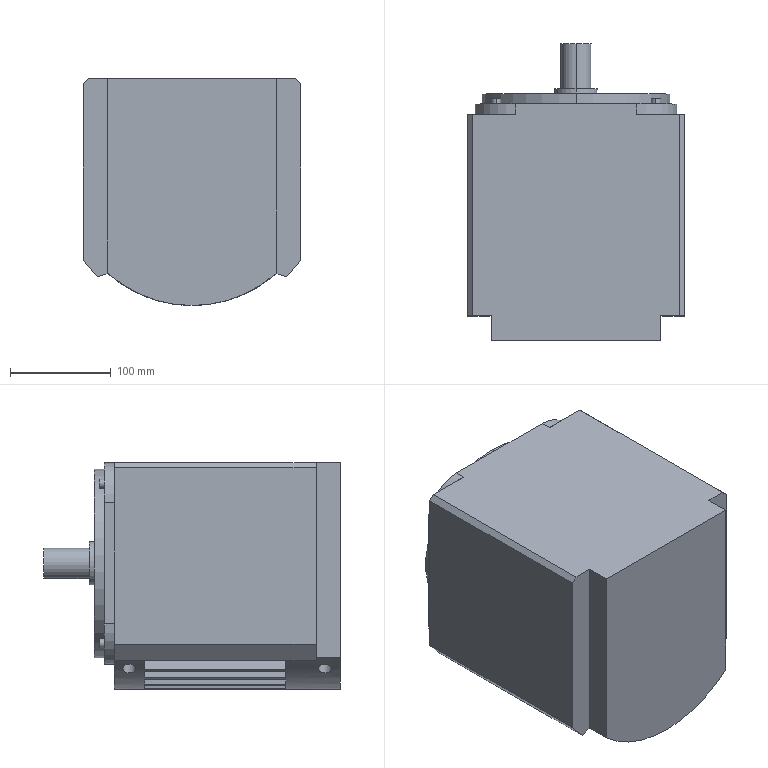Part | SolidWorks | features ICE 13, Chamfer 1, CirPattern 1, Extrusion 1, MirrorPattern 1 | 1 solid | 347 faces | box 215.394 x 294 x 225 mm | volume 10267409 mm3 | plane 235 | cylinder 112 | commonest cylinder face diameters 60 x31 150 x31 220 x12 9 x8 11 x8 13 x8